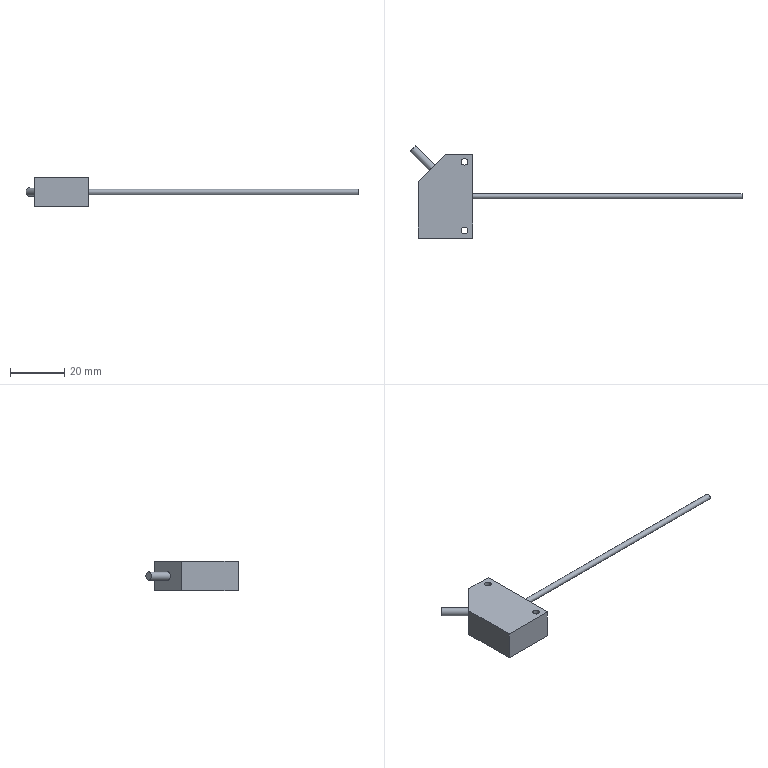Part | NX | 1 solid | 18 faces | box 122.632 x 34.132 x 10.8 mm | volume 6360 mm3 | plane 14 | cylinder 4 | commonest cylinder face diameters 2.5 x2 2 x1 3 x1
STEP:
#1=CARTESIAN_POINT('',(17.5,-33.25,8.4));
#2=VERTEX_POINT('',#1);
#3=CARTESIAN_POINT('',(17.5,-58.25,8.4));
#4=VERTEX_POINT('',#3);
#5=CARTESIAN_POINT('',(17.5,-33.25,8.4));
#6=DIRECTION('',(0.,-1.,0.));
#7=VECTOR('',#6,1000.);
#8=LINE('',#5,#7);
#9=EDGE_CURVE('',#2,#4,#8,.T.);
#10=ORIENTED_EDGE('',*,*,#9,.T.);
#11=CARTESIAN_POINT('',(17.5,-58.25,2.4));
#12=VERTEX_POINT('',#11);
#13=CARTESIAN_POINT('',(17.5,-58.25,8.4));
#14=DIRECTION('',(0.,0.,-1.));
#15=VECTOR('',#14,1000.);
#16=LINE('',#13,#15);
#17=EDGE_CURVE('',#4,#12,#16,.T.);
#18=ORIENTED_EDGE('',*,*,#17,.T.);
#19=CARTESIAN_POINT('',(17.5,-33.25,2.4));
#20=VERTEX_POINT('',#19);
#21=CARTESIAN_POINT('',(17.5,-33.25,2.4));
#22=DIRECTION('',(0.,1.,0.));
#23=VECTOR('',#22,1000.);
#24=LINE('',#21,#23);
#25=EDGE_CURVE('',#12,#20,#24,.T.);
#26=ORIENTED_EDGE('',*,*,#25,.T.);
#27=CARTESIAN_POINT('',(17.5,-33.25,8.4));
#28=DIRECTION('',(0.,0.,1.));
#29=VECTOR('',#28,1000.);
#30=LINE('',#27,#29);
#31=EDGE_CURVE('',#20,#2,#30,.T.);
#32=ORIENTED_EDGE('',*,*,#31,.T.);
#33=EDGE_LOOP('',(#10,#18,#26,#32));
#34=FACE_BOUND('',#33,.T.);
#35=CARTESIAN_POINT('',(17.5,-45.75,4.4));
#36=VERTEX_POINT('',#35);
#37=CARTESIAN_POINT('',(17.5,-45.75,5.4));
#38=DIRECTION('',(1.,0.,0.));
#39=DIRECTION('',(0.,0.,-1.));
#40=AXIS2_PLACEMENT_3D('',#37,#38,#39);
#41=CIRCLE('',#40,1.);
#42=EDGE_CURVE('',#36,#36,#41,.T.);
#43=ORIENTED_EDGE('',*,*,#42,.F.);
#44=EDGE_LOOP('',(#43));
#45=FACE_BOUND('',#44,.T.);
#46=CARTESIAN_POINT('',(17.5,-58.25,8.4));
#47=DIRECTION('',(1.,0.,0.));
#48=DIRECTION('',(0.,0.,-1.));
#49=AXIS2_PLACEMENT_3D('',#46,#47,#48);
#50=PLANE('',#49);
#51=ADVANCED_FACE('',(#34,#45),#50,.T.);
#52=CARTESIAN_POINT('',(8.,-30.25,10.8));
#53=VERTEX_POINT('',#52);
#54=CARTESIAN_POINT('',(-2.,-40.25,10.8));
#55=VERTEX_POINT('',#54);
#56=CARTESIAN_POINT('',(-2.,-40.25,10.8));
#57=DIRECTION('',(0.7071,0.7071,0.));
#58=VECTOR('',#57,1000.);
#59=LINE('',#56,#58);
#60=EDGE_CURVE('',#53,#55,#59,.F.);
#61=ORIENTED_EDGE('',*,*,#60,.F.);
#62=CARTESIAN_POINT('',(8.,-30.25,0.));
#63=VERTEX_POINT('',#62);
#64=CARTESIAN_POINT('',(8.,-30.25,10.8));
#65=DIRECTION('',(0.,0.,1.));
#66=VECTOR('',#65,1000.);
#67=LINE('',#64,#66);
#68=EDGE_CURVE('',#63,#53,#67,.T.);
#69=ORIENTED_EDGE('',*,*,#68,.F.);
#70=CARTESIAN_POINT('',(-2.,-40.25,0.));
#71=VERTEX_POINT('',#70);
#72=CARTESIAN_POINT('',(-2.5,-40.75,0.));
#73=DIRECTION('',(-0.7071,-0.7071,0.));
#74=VECTOR('',#73,1000.);
#75=LINE('',#72,#74);
#76=EDGE_CURVE('',#71,#63,#75,.F.);
#77=ORIENTED_EDGE('',*,*,#76,.F.);
#78=CARTESIAN_POINT('',(-2.,-40.25,10.8));
#79=DIRECTION('',(0.,0.,-1.));
#80=VECTOR('',#79,1000.);
#81=LINE('',#78,#80);
#82=EDGE_CURVE('',#55,#71,#81,.T.);
#83=ORIENTED_EDGE('',*,*,#82,.F.);
#84=EDGE_LOOP('',(#61,#69,#77,#83));
#85=FACE_BOUND('',#84,.T.);
#86=CARTESIAN_POINT('',(1.939,-36.311,5.4));
#87=VERTEX_POINT('',#86);
#88=CARTESIAN_POINT('',(3.,-35.25,5.4));
#89=DIRECTION('',(-0.7071,0.7071,0.));
#90=DIRECTION('',(-0.7071,-0.7071,0.));
#91=AXIS2_PLACEMENT_3D('',#88,#89,#90);
#92=CIRCLE('',#91,1.5);
#93=EDGE_CURVE('',#87,#87,#92,.T.);
#94=ORIENTED_EDGE('',*,*,#93,.F.);
#95=EDGE_LOOP('',(#94));
#96=FACE_BOUND('',#95,.T.);
#97=CARTESIAN_POINT('',(-2.,-40.25,10.8));
#98=DIRECTION('',(0.7071,-0.7071,0.));
#99=DIRECTION('',(0.7071,0.7071,0.));
#100=AXIS2_PLACEMENT_3D('',#97,#98,#99);
#101=PLANE('',#100);
#102=ADVANCED_FACE('',(#85,#96),#101,.F.);
#103=CARTESIAN_POINT('',(18.,-58.25,8.4));
#104=VERTEX_POINT('',#103);
#105=CARTESIAN_POINT('',(18.,-58.25,2.4));
#106=VERTEX_POINT('',#105);
#107=CARTESIAN_POINT('',(18.,-58.25,8.4));
#108=DIRECTION('',(0.,0.,-1.));
#109=VECTOR('',#108,1000.);
#110=LINE('',#107,#109);
#111=EDGE_CURVE('',#104,#106,#110,.T.);
#112=ORIENTED_EDGE('',*,*,#111,.F.);
#113=CARTESIAN_POINT('',(18.,-33.25,8.4));
#114=VERTEX_POINT('',#113);
#115=CARTESIAN_POINT('',(18.,-33.25,8.4));
#116=DIRECTION('',(0.,-1.,0.));
#117=VECTOR('',#116,1000.);
#118=LINE('',#115,#117);
#119=EDGE_CURVE('',#114,#104,#118,.T.);
#120=ORIENTED_EDGE('',*,*,#119,.F.);
#121=CARTESIAN_POINT('',(18.,-33.25,2.4));
#122=VERTEX_POINT('',#121);
#123=CARTESIAN_POINT('',(18.,-33.25,8.4));
#124=DIRECTION('',(0.,0.,1.));
#125=VECTOR('',#124,1000.);
#126=LINE('',#123,#125);
#127=EDGE_CURVE('',#122,#114,#126,.T.);
#128=ORIENTED_EDGE('',*,*,#127,.F.);
#129=CARTESIAN_POINT('',(18.,-33.25,2.4));
#130=DIRECTION('',(0.,1.,0.));
#131=VECTOR('',#130,1000.);
#132=LINE('',#129,#131);
#133=EDGE_CURVE('',#106,#122,#132,.T.);
#134=ORIENTED_EDGE('',*,*,#133,.F.);
#135=EDGE_LOOP('',(#112,#120,#128,#134));
#136=FACE_BOUND('',#135,.T.);
#137=CARTESIAN_POINT('',(18.,-61.25,0.));
#138=VERTEX_POINT('',#137);
#139=CARTESIAN_POINT('',(18.,-30.25,0.));
#140=VERTEX_POINT('',#139);
#141=CARTESIAN_POINT('',(18.,-30.25,0.));
#142=DIRECTION('',(0.,1.,0.));
#143=VECTOR('',#142,1000.);
#144=LINE('',#141,#143);
#145=EDGE_CURVE('',#138,#140,#144,.T.);
#146=ORIENTED_EDGE('',*,*,#145,.T.);
#147=CARTESIAN_POINT('',(18.,-30.25,10.8));
#148=VERTEX_POINT('',#147);
#149=CARTESIAN_POINT('',(18.,-30.25,10.8));
#150=DIRECTION('',(0.,0.,-1.));
#151=VECTOR('',#150,1000.);
#152=LINE('',#149,#151);
#153=EDGE_CURVE('',#148,#140,#152,.T.);
#154=ORIENTED_EDGE('',*,*,#153,.F.);
#155=CARTESIAN_POINT('',(18.,-61.25,10.8));
#156=VERTEX_POINT('',#155);
#157=CARTESIAN_POINT('',(18.,-30.25,10.8));
#158=DIRECTION('',(0.,1.,0.));
#159=VECTOR('',#158,1000.);
#160=LINE('',#157,#159);
#161=EDGE_CURVE('',#156,#148,#160,.T.);
#162=ORIENTED_EDGE('',*,*,#161,.F.);
#163=CARTESIAN_POINT('',(18.,-61.25,10.8));
#164=DIRECTION('',(0.,0.,-1.));
#165=VECTOR('',#164,1000.);
#166=LINE('',#163,#165);
#167=EDGE_CURVE('',#156,#138,#166,.T.);
#168=ORIENTED_EDGE('',*,*,#167,.T.);
#169=EDGE_LOOP('',(#146,#154,#162,#168));
#170=FACE_BOUND('',#169,.T.);
#171=CARTESIAN_POINT('',(18.,-30.25,10.8));
#172=DIRECTION('',(-1.,0.,0.));
#173=DIRECTION('',(0.,0.,1.));
#174=AXIS2_PLACEMENT_3D('',#171,#172,#173);
#175=PLANE('',#174);
#176=ADVANCED_FACE('',(#136,#170),#175,.F.);
#177=CARTESIAN_POINT('',(18.,-30.25,0.));
#178=DIRECTION('',(-1.,0.,0.));
#179=VECTOR('',#178,1000.);
#180=LINE('',#177,#179);
#181=EDGE_CURVE('',#140,#63,#180,.T.);
#182=ORIENTED_EDGE('',*,*,#181,.T.);
#183=ORIENTED_EDGE('',*,*,#68,.T.);
#184=CARTESIAN_POINT('',(18.,-30.25,10.8));
#185=DIRECTION('',(-1.,0.,0.));
#186=VECTOR('',#185,1000.);
#187=LINE('',#184,#186);
#188=EDGE_CURVE('',#148,#53,#187,.T.);
#189=ORIENTED_EDGE('',*,*,#188,.F.);
#190=ORIENTED_EDGE('',*,*,#153,.T.);
#191=EDGE_LOOP('',(#182,#183,#189,#190));
#192=FACE_BOUND('',#191,.T.);
#193=CARTESIAN_POINT('',(18.,-30.25,10.8));
#194=DIRECTION('',(0.,-1.,0.));
#195=DIRECTION('',(1.,0.,0.));
#196=AXIS2_PLACEMENT_3D('',#193,#194,#195);
#197=PLANE('',#196);
#198=ADVANCED_FACE('',(#192),#197,.F.);
#199=CARTESIAN_POINT('',(-2.,-61.25,10.8));
#200=VERTEX_POINT('',#199);
#201=CARTESIAN_POINT('',(-2.,-30.25,10.8));
#202=DIRECTION('',(0.,-1.,0.));
#203=VECTOR('',#202,1000.);
#204=LINE('',#201,#203);
#205=EDGE_CURVE('',#55,#200,#204,.T.);
#206=ORIENTED_EDGE('',*,*,#205,.F.);
#207=ORIENTED_EDGE('',*,*,#82,.T.);
#208=CARTESIAN_POINT('',(-2.,-61.25,0.));
#209=VERTEX_POINT('',#208);
#210=CARTESIAN_POINT('',(-2.,-30.25,0.));
#211=DIRECTION('',(0.,-1.,0.));
#212=VECTOR('',#211,1000.);
#213=LINE('',#210,#212);
#214=EDGE_CURVE('',#71,#209,#213,.T.);
#215=ORIENTED_EDGE('',*,*,#214,.T.);
#216=CARTESIAN_POINT('',(-2.,-61.25,10.8));
#217=DIRECTION('',(0.,0.,-1.));
#218=VECTOR('',#217,1000.);
#219=LINE('',#216,#218);
#220=EDGE_CURVE('',#200,#209,#219,.T.);
#221=ORIENTED_EDGE('',*,*,#220,.F.);
#222=EDGE_LOOP('',(#206,#207,#215,#221));
#223=FACE_BOUND('',#222,.T.);
#224=CARTESIAN_POINT('',(-2.,-30.25,10.8));
#225=DIRECTION('',(1.,0.,0.));
#226=DIRECTION('',(0.,1.,0.));
#227=AXIS2_PLACEMENT_3D('',#224,#225,#226);
#228=PLANE('',#227);
#229=ADVANCED_FACE('',(#223),#228,.F.);
#230=CARTESIAN_POINT('',(18.,-61.25,0.));
#231=DIRECTION('',(1.,0.,0.));
#232=VECTOR('',#231,1000.);
#233=LINE('',#230,#232);
#234=EDGE_CURVE('',#209,#138,#233,.T.);
#235=ORIENTED_EDGE('',*,*,#234,.T.);
#236=ORIENTED_EDGE('',*,*,#167,.F.);
#237=CARTESIAN_POINT('',(18.,-61.25,10.8));
#238=DIRECTION('',(1.,0.,0.));
#239=VECTOR('',#238,1000.);
#240=LINE('',#237,#239);
#241=EDGE_CURVE('',#200,#156,#240,.T.);
#242=ORIENTED_EDGE('',*,*,#241,.F.);
#243=ORIENTED_EDGE('',*,*,#220,.T.);
#244=EDGE_LOOP('',(#235,#236,#242,#243));
#245=FACE_BOUND('',#244,.T.);
#246=CARTESIAN_POINT('',(18.,-61.25,10.8));
#247=DIRECTION('',(0.,1.,0.));
#248=DIRECTION('',(-1.,0.,0.));
#249=AXIS2_PLACEMENT_3D('',#246,#247,#248);
#250=PLANE('',#249);
#251=ADVANCED_FACE('',(#245),#250,.F.);
#252=CARTESIAN_POINT('',(16.25,-58.45,10.8));
#253=VERTEX_POINT('',#252);
#254=CARTESIAN_POINT('',(15.,-58.45,10.8));
#255=DIRECTION('',(0.,0.,1.));
#256=DIRECTION('',(1.,0.,0.));
#257=AXIS2_PLACEMENT_3D('',#254,#255,#256);
#258=CIRCLE('',#257,1.25);
#259=EDGE_CURVE('',#253,#253,#258,.T.);
#260=ORIENTED_EDGE('',*,*,#259,.F.);
#261=EDGE_LOOP('',(#260));
#262=FACE_BOUND('',#261,.T.);
#263=CARTESIAN_POINT('',(16.25,-33.05,10.8));
#264=VERTEX_POINT('',#263);
#265=CARTESIAN_POINT('',(15.,-33.05,10.8));
#266=DIRECTION('',(0.,0.,1.));
#267=DIRECTION('',(1.,0.,0.));
#268=AXIS2_PLACEMENT_3D('',#265,#266,#267);
#269=CIRCLE('',#268,1.25);
#270=EDGE_CURVE('',#264,#264,#269,.T.);
#271=ORIENTED_EDGE('',*,*,#270,.F.);
#272=EDGE_LOOP('',(#271));
#273=FACE_BOUND('',#272,.T.);
#274=ORIENTED_EDGE('',*,*,#188,.T.);
#275=ORIENTED_EDGE('',*,*,#60,.T.);
#276=ORIENTED_EDGE('',*,*,#205,.T.);
#277=ORIENTED_EDGE('',*,*,#241,.T.);
#278=ORIENTED_EDGE('',*,*,#161,.T.);
#279=EDGE_LOOP('',(#274,#275,#276,#277,#278));
#280=FACE_BOUND('',#279,.T.);
#281=CARTESIAN_POINT('',(18.,-61.25,10.8));
#282=DIRECTION('',(0.,0.,-1.));
#283=DIRECTION('',(-1.,0.,0.));
#284=AXIS2_PLACEMENT_3D('',#281,#282,#283);
#285=PLANE('',#284);
#286=ADVANCED_FACE('',(#262,#273,#280),#285,.F.);
#287=CARTESIAN_POINT('',(16.25,-58.45,0.));
#288=VERTEX_POINT('',#287);
#289=CARTESIAN_POINT('',(15.,-58.45,0.));
#290=DIRECTION('',(0.,0.,1.));
#291=DIRECTION('',(1.,0.,0.));
#292=AXIS2_PLACEMENT_3D('',#289,#290,#291);
#293=CIRCLE('',#292,1.25);
#294=EDGE_CURVE('',#288,#288,#293,.T.);
#295=ORIENTED_EDGE('',*,*,#294,.T.);
#296=EDGE_LOOP('',(#295));
#297=FACE_BOUND('',#296,.T.);
#298=CARTESIAN_POINT('',(16.25,-33.05,0.));
#299=VERTEX_POINT('',#298);
#300=CARTESIAN_POINT('',(15.,-33.05,0.));
#301=DIRECTION('',(0.,0.,1.));
#302=DIRECTION('',(1.,0.,0.));
#303=AXIS2_PLACEMENT_3D('',#300,#301,#302);
#304=CIRCLE('',#303,1.25);
#305=EDGE_CURVE('',#299,#299,#304,.T.);
#306=ORIENTED_EDGE('',*,*,#305,.T.);
#307=EDGE_LOOP('',(#306));
#308=FACE_BOUND('',#307,.T.);
#309=ORIENTED_EDGE('',*,*,#214,.F.);
#310=ORIENTED_EDGE('',*,*,#76,.T.);
#311=ORIENTED_EDGE('',*,*,#181,.F.);
#312=ORIENTED_EDGE('',*,*,#145,.F.);
#313=ORIENTED_EDGE('',*,*,#234,.F.);
#314=EDGE_LOOP('',(#309,#310,#311,#312,#313));
#315=FACE_BOUND('',#314,.T.);
#316=CARTESIAN_POINT('',(18.,-61.25,0.));
#317=DIRECTION('',(0.,0.,-1.));
#318=DIRECTION('',(-1.,0.,0.));
#319=AXIS2_PLACEMENT_3D('',#316,#317,#318);
#320=PLANE('',#319);
#321=ADVANCED_FACE('',(#297,#308,#315),#320,.T.);
#322=CARTESIAN_POINT('',(-5.132,-29.24,5.4));
#323=VERTEX_POINT('',#322);
#324=CARTESIAN_POINT('',(-4.071,-28.179,5.4));
#325=DIRECTION('',(-0.7071,0.7071,0.));
#326=DIRECTION('',(-0.7071,-0.7071,0.));
#327=AXIS2_PLACEMENT_3D('',#324,#325,#326);
#328=CIRCLE('',#327,1.5);
#329=EDGE_CURVE('',#323,#323,#328,.T.);
#330=ORIENTED_EDGE('',*,*,#329,.F.);
#331=EDGE_LOOP('',(#330));
#332=FACE_BOUND('',#331,.T.);
#333=ORIENTED_EDGE('',*,*,#93,.T.);
#334=EDGE_LOOP('',(#333));
#335=FACE_BOUND('',#334,.T.);
#336=CARTESIAN_POINT('',(-4.071,-28.179,5.4));
#337=DIRECTION('',(0.7071,-0.7071,0.));
#338=DIRECTION('',(0.7071,0.7071,0.));
#339=AXIS2_PLACEMENT_3D('',#336,#337,#338);
#340=CYLINDRICAL_SURFACE('',#339,1.5);
#341=ADVANCED_FACE('',(#332,#335),#340,.T.);
#342=ORIENTED_EDGE('',*,*,#329,.T.);
#343=EDGE_LOOP('',(#342));
#344=FACE_BOUND('',#343,.T.);
#345=CARTESIAN_POINT('',(-4.071,-28.179,5.4));
#346=DIRECTION('',(-0.7071,0.7071,0.));
#347=DIRECTION('',(-0.7071,-0.7071,0.));
#348=AXIS2_PLACEMENT_3D('',#345,#346,#347);
#349=PLANE('',#348);
#350=ADVANCED_FACE('',(#344),#349,.T.);
#351=ORIENTED_EDGE('',*,*,#305,.F.);
#352=EDGE_LOOP('',(#351));
#353=FACE_BOUND('',#352,.T.);
#354=ORIENTED_EDGE('',*,*,#270,.T.);
#355=EDGE_LOOP('',(#354));
#356=FACE_BOUND('',#355,.T.);
#357=CARTESIAN_POINT('',(15.,-33.05,10.8));
#358=DIRECTION('',(0.,0.,1.));
#359=DIRECTION('',(1.,0.,0.));
#360=AXIS2_PLACEMENT_3D('',#357,#358,#359);
#361=CYLINDRICAL_SURFACE('',#360,1.25);
#362=ADVANCED_FACE('',(#353,#356),#361,.F.);
#363=ORIENTED_EDGE('',*,*,#294,.F.);
#364=EDGE_LOOP('',(#363));
#365=FACE_BOUND('',#364,.T.);
#366=ORIENTED_EDGE('',*,*,#259,.T.);
#367=EDGE_LOOP('',(#366));
#368=FACE_BOUND('',#367,.T.);
#369=CARTESIAN_POINT('',(15.,-58.45,10.8));
#370=DIRECTION('',(0.,0.,1.));
#371=DIRECTION('',(1.,0.,0.));
#372=AXIS2_PLACEMENT_3D('',#369,#370,#371);
#373=CYLINDRICAL_SURFACE('',#372,1.25);
#374=ADVANCED_FACE('',(#365,#368),#373,.F.);
#375=ORIENTED_EDGE('',*,*,#119,.T.);
#376=CARTESIAN_POINT('',(17.5,-58.25,8.4));
#377=DIRECTION('',(1.,0.,0.));
#378=VECTOR('',#377,1000.);
#379=LINE('',#376,#378);
#380=EDGE_CURVE('',#4,#104,#379,.T.);
#381=ORIENTED_EDGE('',*,*,#380,.F.);
#382=ORIENTED_EDGE('',*,*,#9,.F.);
#383=CARTESIAN_POINT('',(17.5,-33.25,8.4));
#384=DIRECTION('',(1.,0.,0.));
#385=VECTOR('',#384,1000.);
#386=LINE('',#383,#385);
#387=EDGE_CURVE('',#2,#114,#386,.T.);
#388=ORIENTED_EDGE('',*,*,#387,.T.);
#389=EDGE_LOOP('',(#375,#381,#382,#388));
#390=FACE_BOUND('',#389,.T.);
#391=CARTESIAN_POINT('',(17.5,-33.25,8.4));
#392=DIRECTION('',(0.,0.,1.));
#393=DIRECTION('',(0.,-1.,0.));
#394=AXIS2_PLACEMENT_3D('',#391,#392,#393);
#395=PLANE('',#394);
#396=ADVANCED_FACE('',(#390),#395,.F.);
#397=ORIENTED_EDGE('',*,*,#127,.T.);
#398=ORIENTED_EDGE('',*,*,#387,.F.);
#399=ORIENTED_EDGE('',*,*,#31,.F.);
#400=CARTESIAN_POINT('',(17.5,-33.25,2.4));
#401=DIRECTION('',(1.,0.,0.));
#402=VECTOR('',#401,1000.);
#403=LINE('',#400,#402);
#404=EDGE_CURVE('',#20,#122,#403,.T.);
#405=ORIENTED_EDGE('',*,*,#404,.T.);
#406=EDGE_LOOP('',(#397,#398,#399,#405));
#407=FACE_BOUND('',#406,.T.);
#408=CARTESIAN_POINT('',(17.5,-33.25,8.4));
#409=DIRECTION('',(0.,1.,0.));
#410=DIRECTION('',(0.,0.,1.));
#411=AXIS2_PLACEMENT_3D('',#408,#409,#410);
#412=PLANE('',#411);
#413=ADVANCED_FACE('',(#407),#412,.F.);
#414=ORIENTED_EDGE('',*,*,#133,.T.);
#415=ORIENTED_EDGE('',*,*,#404,.F.);
#416=ORIENTED_EDGE('',*,*,#25,.F.);
#417=CARTESIAN_POINT('',(17.5,-58.25,2.4));
#418=DIRECTION('',(1.,0.,0.));
#419=VECTOR('',#418,1000.);
#420=LINE('',#417,#419);
#421=EDGE_CURVE('',#12,#106,#420,.T.);
#422=ORIENTED_EDGE('',*,*,#421,.T.);
#423=EDGE_LOOP('',(#414,#415,#416,#422));
#424=FACE_BOUND('',#423,.T.);
#425=CARTESIAN_POINT('',(17.5,-33.25,2.4));
#426=DIRECTION('',(0.,0.,-1.));
#427=DIRECTION('',(0.,1.,0.));
#428=AXIS2_PLACEMENT_3D('',#425,#426,#427);
#429=PLANE('',#428);
#430=ADVANCED_FACE('',(#424),#429,.F.);
#431=ORIENTED_EDGE('',*,*,#111,.T.);
#432=ORIENTED_EDGE('',*,*,#421,.F.);
#433=ORIENTED_EDGE('',*,*,#17,.F.);
#434=ORIENTED_EDGE('',*,*,#380,.T.);
#435=EDGE_LOOP('',(#431,#432,#433,#434));
#436=FACE_BOUND('',#435,.T.);
#437=CARTESIAN_POINT('',(17.5,-58.25,8.4));
#438=DIRECTION('',(0.,-1.,0.));
#439=DIRECTION('',(0.,0.,-1.));
#440=AXIS2_PLACEMENT_3D('',#437,#438,#439);
#441=PLANE('',#440);
#442=ADVANCED_FACE('',(#436),#441,.F.);
#443=CARTESIAN_POINT('',(117.5,-45.75,4.4));
#444=VERTEX_POINT('',#443);
#445=CARTESIAN_POINT('',(117.5,-45.75,5.4));
#446=DIRECTION('',(1.,0.,0.));
#447=DIRECTION('',(0.,0.,-1.));
#448=AXIS2_PLACEMENT_3D('',#445,#446,#447);
#449=CIRCLE('',#448,1.);
#450=EDGE_CURVE('',#444,#444,#449,.T.);
#451=ORIENTED_EDGE('',*,*,#450,.F.);
#452=EDGE_LOOP('',(#451));
#453=FACE_BOUND('',#452,.T.);
#454=ORIENTED_EDGE('',*,*,#42,.T.);
#455=EDGE_LOOP('',(#454));
#456=FACE_BOUND('',#455,.T.);
#457=CARTESIAN_POINT('',(117.5,-45.75,5.4));
#458=DIRECTION('',(-1.,0.,0.));
#459=DIRECTION('',(0.,0.,1.));
#460=AXIS2_PLACEMENT_3D('',#457,#458,#459);
#461=CYLINDRICAL_SURFACE('',#460,1.);
#462=ADVANCED_FACE('',(#453,#456),#461,.T.);
#463=ORIENTED_EDGE('',*,*,#450,.T.);
#464=EDGE_LOOP('',(#463));
#465=FACE_BOUND('',#464,.T.);
#466=CARTESIAN_POINT('',(117.5,-45.75,5.4));
#467=DIRECTION('',(1.,0.,0.));
#468=DIRECTION('',(0.,0.,-1.));
#469=AXIS2_PLACEMENT_3D('',#466,#467,#468);
#470=PLANE('',#469);
#471=ADVANCED_FACE('',(#465),#470,.T.);
#472=CLOSED_SHELL('',(#51,#102,#176,#198,#229,#251,#286,#321,#341,#350,#362,#374,#396,#413,#430,#442,#462,#471));
#473=MANIFOLD_SOLID_BREP('',#472);
#474=(LENGTH_UNIT()NAMED_UNIT(*)SI_UNIT(.MILLI.,.METRE.));
#475=UNCERTAINTY_MEASURE_WITH_UNIT(LENGTH_MEASURE(0.00001),#474,'','');
#476=(NAMED_UNIT(*)PLANE_ANGLE_UNIT()SI_UNIT($,.RADIAN.));
#477=(NAMED_UNIT(*)SI_UNIT($,.STERADIAN.)SOLID_ANGLE_UNIT());
#478=(GEOMETRIC_REPRESENTATION_CONTEXT(3)GLOBAL_UNCERTAINTY_ASSIGNED_CONTEXT((#475))GLOBAL_UNIT_ASSIGNED_CONTEXT((#474,#476,#477))REPRESENTATION_CONTEXT('',''));
#479=ADVANCED_BREP_SHAPE_REPRESENTATION('',(#473),#478);